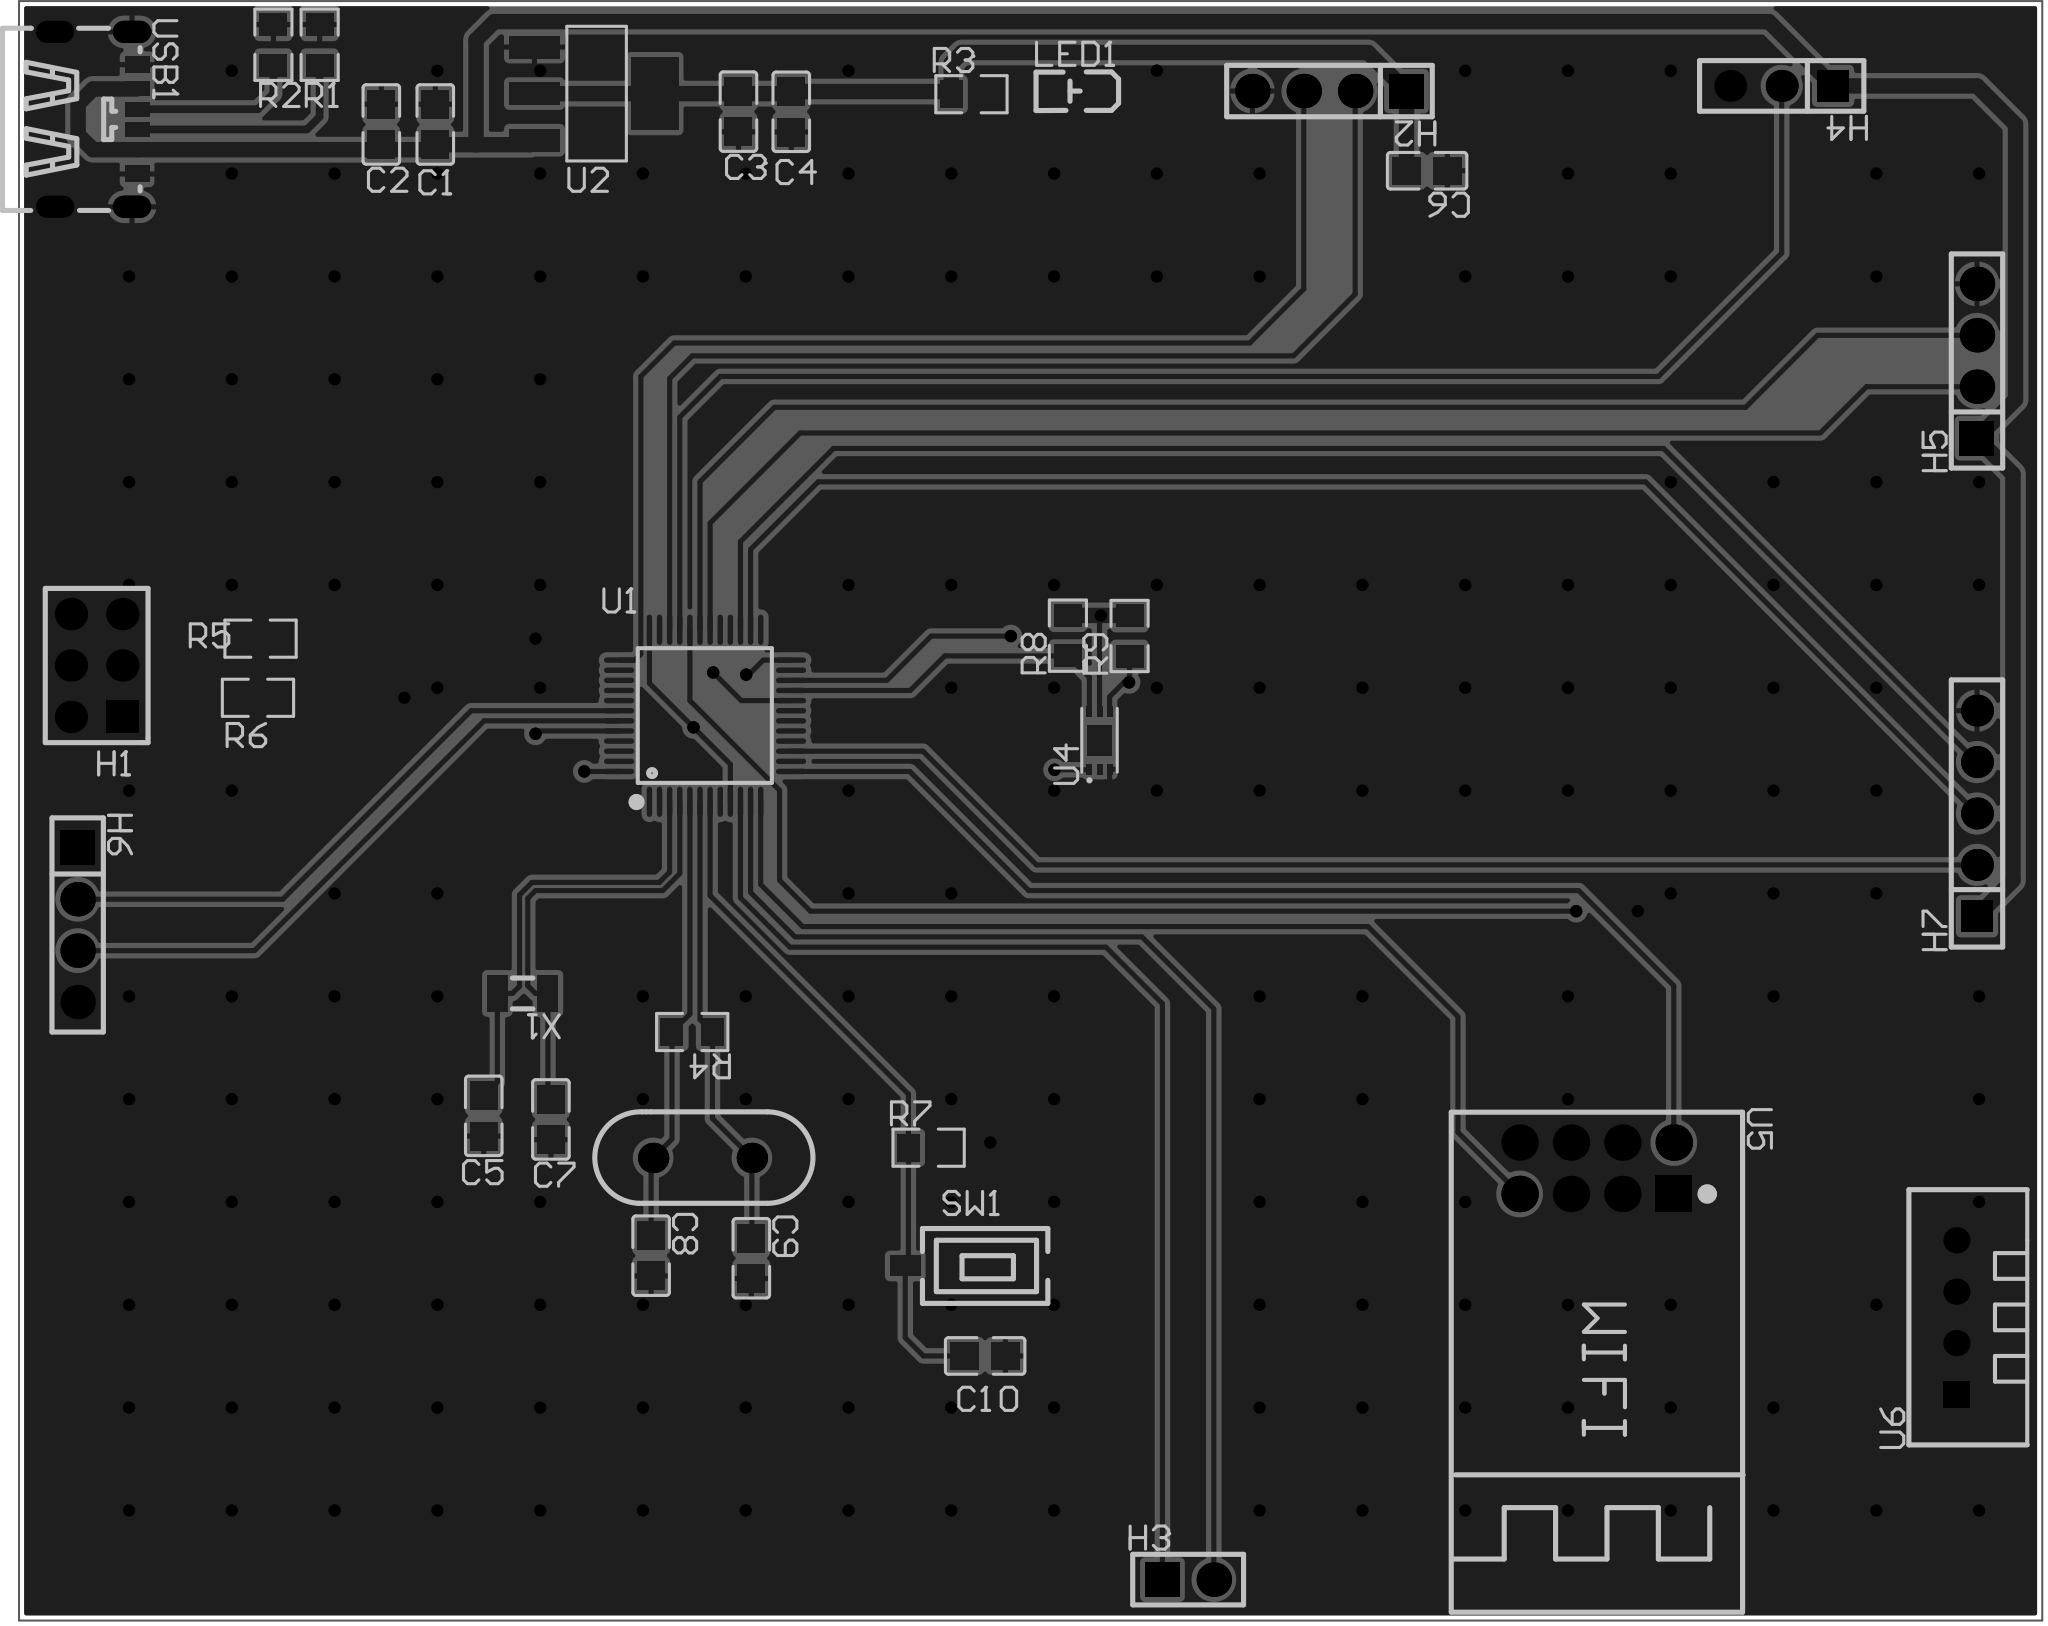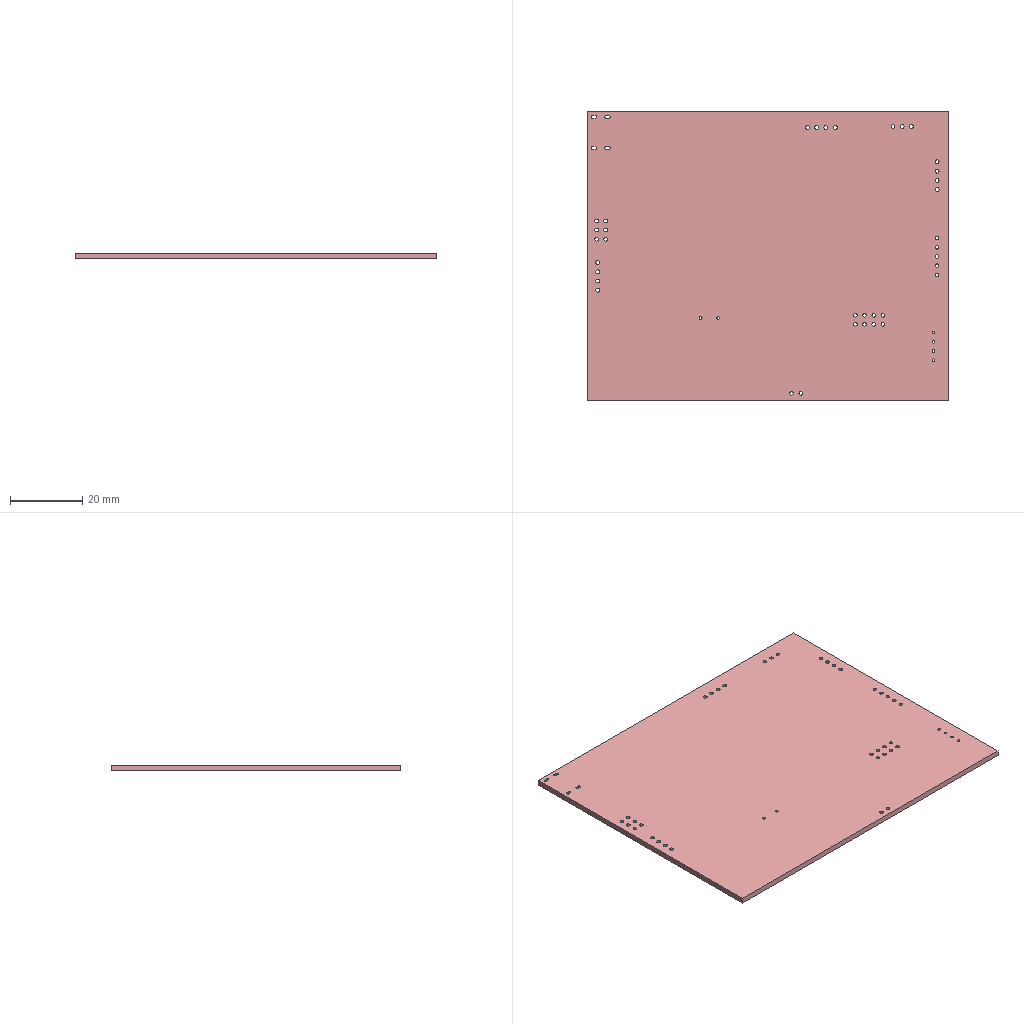Circuit board layout | Altium Designer | box 100 x 80 x 1.6 mm
Layer stack:
# Altium Designer layer stack of  (unit mm; dielectric type: 0 none, 1 core, 2 prepreg, 3 surface material)
index,name,kind,layer,copper_thickness_mm,dielectric_type,dielectric_thickness_mm,dielectric_material,dielectric_constant
0,Top Paste Mask Layer,other,,,,,,
1,Top Silkscreen Layer,other,,,,,,
2,Top Solder Mask Layer,dielectric,,,3,0.01,,3.3
3,Top Layer,copper,Top Layer,0.035,,,,
4,Dielectric1,dielectric,,,3,1.51,FR4,4.5
5,Bottom Layer,copper,Bottom Layer,0.035,,,,
6,Bottom Solder Mask Layer,dielectric,,,3,0.01,,3.3
7,Bottom Silkscreen Layer,other,,,,,,
8,Bottom Paste Mask Layer,other,,,,,,
# drill layer pairs: low layer,high layer
drill_pair,Top Layer,Bottom Layer
Part placement:
Designator,Comment,Layer,Footprint,Center-X(mm),Center-Y(mm),Rotation
C1,100nF,TopLayer,C0805,110.998,157.734,270
C2,10uF,TopLayer,C0805,108.331,157.734,270
C3,100nF,TopLayer,C0805,125.984,158.369,90
C4,10uF,TopLayer,C0805,128.593,158.361,90
C5,20PF,TopLayer,C0805,113.395,108.762,270
C6,100nF,TopLayer,C0805,160.02,155.448,180
C7,20PF,TopLayer,C0805,116.713,108.585,90
C8,20PF,TopLayer,C0805,121.666,101.854,270
C9,20PF,TopLayer,C0805,126.619,101.727,270
C10,100nF,TopLayer,C0805,138.176,96.901,180
H1,,TopLayer,HDR-TH_6P-P2.54-V-R2-C3-S2.54_A2541WV-2X3P,94.261,131.007,90
H2,,TopLayer,HDR-TH_4P-P2.54-V-M,155.194,159.385,180
H3,,TopLayer,HDR-TH_2P-P2.54-V-F,148.209,85.852,0
H4,,TopLayer,HDR-TH_3P-P2.54-V-F,177.546,159.639,180
H5,,TopLayer,HDR-TH_4P-P2.54-V-F,187.198,146.05,90
H6,,TopLayer,HDR-TH_4P-P2.54-V-F,93.323,118.191,270
H7,,TopLayer,HDR-TH_5P-P2.54-V-F,187.198,123.698,90
LED1,,TopLayer,LED_0805,142.671,159.38,180
R1,5.1k,TopLayer,R0805,105.283,161.671,90
R2,5.1k,TopLayer,R0805,102.997,161.671,90
R3,1K,TopLayer,R0805,137.499,159.228,0
R4,1M,TopLayer,R0805,123.698,112.903,180
R5,10K,TopLayer,R0805,102.362,132.334,0
R6,10K,TopLayer,R0805,102.235,129.413,180
R7,10K,TopLayer,R0805,135.382,107.188,0
R8,10K,TopLayer,R0805,142.266,132.482,90
R9,10K,TopLayer,R0805,145.314,132.466,90
SW1,,TopLayer,Key_SMD_3.6x6.1x2.5,138.176,101.346,180
U1,STM32F103C8T6,TopLayer,LQFP-48_L7.0-W7.0-P0.50-LS9.0-BL,124.333,128.524,0
U2,AMS1117-3.3,TopLayer,SOT-223-3_L6.5-W3.4-P2.30-LS7.0-BR,118.872,159.258,180
U3,8MHz,TopLayer,CRYSTAL-TH_L10.8-W4.5-P4.88,124.206,106.68,180
U4,BH1750FVI-TR,TopLayer,WSOF-6_L2.6-W1.6-P0.50-TL-EP,143.828,127.314,90
U5,2.4GHz,TopLayer,WIFIM-TH_8P-L24.7-W14.4-P2.54,168.402,106.172,270
U6,DHT11,TopLayer,SENSOR-TH_DHT11,186.182,98.806,90
USB1,TYPE-C-6P-DIP2X2,TopLayer,TYPE-C-SMD_TYPE-C-6P,94.234,157.988,270
X1,32.768kHz,TopLayer,FC-135R_L3.2-W1.5,115.316,114.808,180
Pad and via stacks:
# Altium Designer via and pad stacks of  (unit mm). Each distinct definition once, with the count of objects using it.
# via: kind,start_layer,end_layer,hole_mm,diameter_mm,mode(0 simple;1 top-mid-bottom;2 full stack),diameter_per_layer,count,example_net
# pad: kind,layer,hole_mm,hole_type(0 round;1 square;2 slot),plating,top_size,top_shape(1 round;2 rect;3 octagon;9 rounded rect),mid_size,bottom_size,mode,footprint,size_per_layer,count,example
pad,Top Layer,0,0,plated,1.41x1.35,2,1.41x1.35,1.41x1.35,0,C0805,,20,C1.2
pad,Top Layer,0,0,plated,1x1.25,2,1x1.25,1x1.25,0,LED_0805,,2,LED1.2
pad,Top Layer,0,0,plated,1.133x1.377,2,1.133x1.377,1.133x1.377,0,R0805,,18,R1.2
pad,Top Layer,0,0,plated,1.501x1.001,2,1.501x1.001,1.501x1.001,0,Key_SMD_3.6x6.1x2.5,,2,SW1.2
pad,Top Layer,0,0,plated,0.27x1.5,1,0.27x1.5,0.27x1.5,0,LQFP-48_L7.0-W7.0-P0.50-LS9.0-BL,,24,U1.1
pad,Top Layer,0,0,plated,1.5x0.27,1,1.5x0.27,1.5x0.27,0,LQFP-48_L7.0-W7.0-P0.50-LS9.0-BL,,24,U1.13
pad,Top Layer,0,0,plated,2.5x1.1,2,2.5x1.1,2.5x1.1,0,SOT-223-3_L6.5-W3.4-P2.30-LS7.0-BR,,3,U2.1
pad,Top Layer,0,0,plated,2.34x3.6,2,2.34x3.6,2.34x3.6,0,SOT-223-3_L6.5-W3.4-P2.30-LS7.0-BR,,1,U2.4
pad,Top Layer,0,0,plated,0.505x0.28,2,0.505x0.28,0.505x0.28,0,WSOF-6_L2.6-W1.6-P0.50-TL-EP,,6,U4.1
pad,Top Layer,0,0,plated,1.5x1.2,2,1.5x1.2,1.5x1.2,0,WSOF-6_L2.6-W1.6-P0.50-TL-EP,,1,U4.7
pad,Top Layer,0,0,plated,0.8x1.2,2,0.8x1.2,0.8x1.2,0,TYPE-C-SMD_TYPE-C-6P,,2,USB1.B12
pad,Top Layer,0,0,plated,0.7x1.2,2,0.7x1.2,0.7x1.2,0,TYPE-C-SMD_TYPE-C-6P,,4,USB1.B9
pad,Top Layer,0,0,plated,1.8x1,2,1.8x1,1.8x1,0,FC-135R_L3.2-W1.5,,2,X1.1
pad,Multi-Layer,1.05,0,plated,1.6x1.6,2,1.6x1.6,1.6x1.6,0,HDR-TH_6P-P2.54-V-R2-C3-S2.54_A2541WV-2X3P,,1,H1.1
pad,Multi-Layer,1.05,0,plated,1.6x1.6,1,1.6x1.6,1.6x1.6,0,HDR-TH_6P-P2.54-V-R2-C3-S2.54_A2541WV-2X3P,,5,H1.2
pad,Multi-Layer,1.1,0,plated,1.7x1.7,2,1.7x1.7,1.7x1.7,0,HDR-TH_4P-P2.54-V-M,,1,H2.1
pad,Multi-Layer,1.1,0,plated,1.7x1.7,1,1.7x1.7,1.7x1.7,0,HDR-TH_4P-P2.54-V-M,,3,H2.2
pad,Multi-Layer,1,0,plated,1.7x1.7,2,1.7x1.7,1.7x1.7,0,HDR-TH_2P-P2.54-V-F,,1,H3.1
pad,Multi-Layer,1,0,plated,1.7x1.7,1,1.7x1.7,1.7x1.7,0,HDR-TH_2P-P2.54-V-F,,1,H3.2
pad,Multi-Layer,1.02,0,plated,1.575x1.575,1,1.575x1.575,1.575x1.575,0,HDR-TH_3P-P2.54-V-F,,2,H4.3
pad,Multi-Layer,1.02,0,plated,1.575x1.575,2,1.575x1.575,1.575x1.575,0,HDR-TH_3P-P2.54-V-F,,1,H4.1
pad,Multi-Layer,1.1,0,plated,1.7x1.7,2,1.7x1.7,1.7x1.7,0,HDR-TH_4P-P2.54-V-F,,2,H5.1
pad,Multi-Layer,1.1,0,plated,1.7x1.7,1,1.7x1.7,1.7x1.7,0,HDR-TH_4P-P2.54-V-F,,6,H5.2
pad,Multi-Layer,1.02,0,plated,1.575x1.575,1,1.575x1.575,1.575x1.575,0,HDR-TH_5P-P2.54-V-F,,4,H7.5
pad,Multi-Layer,1.02,0,plated,1.575x1.575,2,1.575x1.575,1.575x1.575,0,HDR-TH_5P-P2.54-V-F,,1,H7.1
pad,Multi-Layer,0.8,0,plated,1.5x1.5,1,1.5x1.5,1.5x1.5,0,CRYSTAL-TH_L10.8-W4.5-P4.88,,2,U3.1
pad,Multi-Layer,1,0,plated,1.8x1.8,1,1.8x1.8,1.8x1.8,0,WIFIM-TH_8P-L24.7-W14.4-P2.54,,7,U5.8
pad,Multi-Layer,1,0,plated,1.8x1.8,2,1.8x1.8,1.8x1.8,0,WIFIM-TH_8P-L24.7-W14.4-P2.54,,1,U5.1
pad,Multi-Layer,0.7112,0,plated,1.295x1.295,2,1.295x1.295,1.295x1.295,0,SENSOR-TH_DHT11,,1,U6.1
pad,Multi-Layer,0.7112,0,plated,1.295x1.295,1,1.295x1.295,1.295x1.295,0,SENSOR-TH_DHT11,,3,U6.2
pad,Multi-Layer,0.7,2,plated,1.1x1.9,1,1.1x1.9,1.1x1.9,0,TYPE-C-SMD_TYPE-C-6P,,4,USB1.7
via,Top Layer,Bottom Layer,0.3048,0.61,0,,204,PB11
Copper pours:
name,layer,net,type(0 solid;1 hatched;2 none)
Bottom Layer-GND,Bottom Layer,GND,0
Top Layer-GND,Top Layer,GND,0